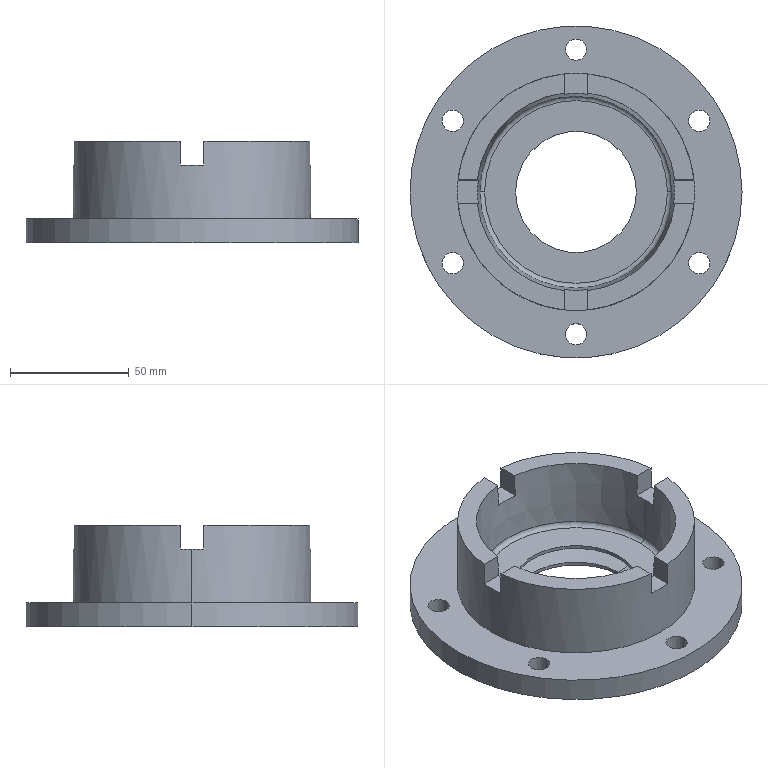Part | SolidWorks | features ICE 6, CirPattern 2, Fillet 1, MirrorPattern 1, RevCut 1, Revolution 1 | 1 solid | 1005 faces | box 140 x 140 x 42.75 mm | volume 195450 mm3 | plane 717 | spline 256 | cylinder 22 | cone 6 | torus 4 | commonest cylinder face diameters 9 x12 51 x4 69 x2 100 x2 140 x2